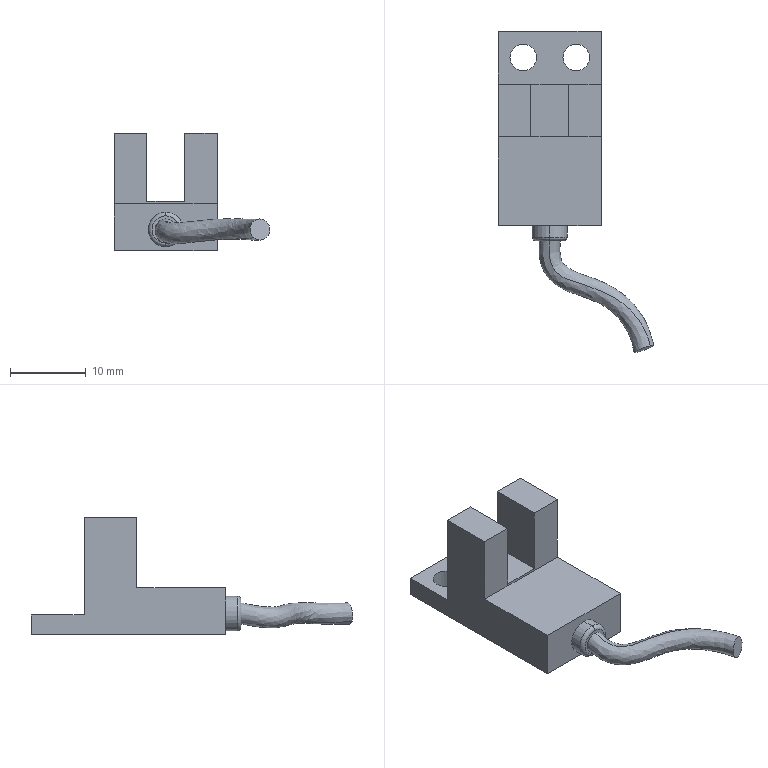Part | SolidWorks | features ICE 5, 3DProfileFeature 2, Extrusion 1, Fillet 1, Sweep 1 | 1 solid | 26 faces | box 20.544 x 42.48 x 15.5 mm | volume 2497 mm3 | plane 16 | cylinder 6 | torus 2 | spline 2 | commonest cylinder face diameters 3.5 x4 4.6 x2
STEP:
#1=CARTESIAN_POINT('',(1.75,9.375,0.));
#2=VERTEX_POINT('',#1);
#3=CARTESIAN_POINT('',(5.25,9.375,0.));
#4=VERTEX_POINT('',#3);
#5=CARTESIAN_POINT('',(3.5,9.375,0.));
#6=DIRECTION('',(0.,0.,1.));
#7=DIRECTION('',(1.,0.,0.));
#8=AXIS2_PLACEMENT_3D('',#5,#6,#7);
#9=CIRCLE('',#8,1.75);
#10=EDGE_CURVE('',#2,#4,#9,.T.);
#11=ORIENTED_EDGE('',*,*,#10,.F.);
#12=CARTESIAN_POINT('',(1.75,9.375,2.6));
#13=VERTEX_POINT('',#12);
#14=CARTESIAN_POINT('',(1.75,9.375,-7.4));
#15=DIRECTION('',(0.,0.,1.));
#16=VECTOR('',#15,1000.);
#17=LINE('',#14,#16);
#18=EDGE_CURVE('',#2,#13,#17,.T.);
#19=ORIENTED_EDGE('',*,*,#18,.T.);
#20=CARTESIAN_POINT('',(5.25,9.375,2.6));
#21=VERTEX_POINT('',#20);
#22=CARTESIAN_POINT('',(3.5,9.375,2.6));
#23=DIRECTION('',(0.,0.,1.));
#24=DIRECTION('',(-1.,0.,0.));
#25=AXIS2_PLACEMENT_3D('',#22,#23,#24);
#26=CIRCLE('',#25,1.75);
#27=EDGE_CURVE('',#13,#21,#26,.T.);
#28=ORIENTED_EDGE('',*,*,#27,.T.);
#29=CARTESIAN_POINT('',(5.25,9.375,-7.4));
#30=DIRECTION('',(0.,0.,1.));
#31=VECTOR('',#30,1000.);
#32=LINE('',#29,#31);
#33=EDGE_CURVE('',#4,#21,#32,.T.);
#34=ORIENTED_EDGE('',*,*,#33,.F.);
#35=EDGE_LOOP('',(#11,#19,#28,#34));
#36=FACE_OUTER_BOUND('',#35,.T.);
#37=CARTESIAN_POINT('',(3.5,9.375,-7.4));
#38=DIRECTION('',(0.,0.,1.));
#39=DIRECTION('',(1.,0.,0.));
#40=AXIS2_PLACEMENT_3D('',#37,#38,#39);
#41=CYLINDRICAL_SURFACE('',#40,1.75);
#42=ADVANCED_FACE('',(#36),#41,.F.);
#43=CARTESIAN_POINT('',(-5.25,9.375,0.));
#44=VERTEX_POINT('',#43);
#45=CARTESIAN_POINT('',(-1.75,9.375,0.));
#46=VERTEX_POINT('',#45);
#47=CARTESIAN_POINT('',(-3.5,9.375,0.));
#48=DIRECTION('',(0.,0.,1.));
#49=DIRECTION('',(1.,0.,0.));
#50=AXIS2_PLACEMENT_3D('',#47,#48,#49);
#51=CIRCLE('',#50,1.75);
#52=EDGE_CURVE('',#44,#46,#51,.T.);
#53=ORIENTED_EDGE('',*,*,#52,.F.);
#54=CARTESIAN_POINT('',(-5.25,9.375,2.6));
#55=VERTEX_POINT('',#54);
#56=CARTESIAN_POINT('',(-5.25,9.375,-7.4));
#57=DIRECTION('',(0.,0.,1.));
#58=VECTOR('',#57,1000.);
#59=LINE('',#56,#58);
#60=EDGE_CURVE('',#44,#55,#59,.T.);
#61=ORIENTED_EDGE('',*,*,#60,.T.);
#62=CARTESIAN_POINT('',(-1.75,9.375,2.6));
#63=VERTEX_POINT('',#62);
#64=CARTESIAN_POINT('',(-3.5,9.375,2.6));
#65=DIRECTION('',(0.,0.,1.));
#66=DIRECTION('',(1.,0.,0.));
#67=AXIS2_PLACEMENT_3D('',#64,#65,#66);
#68=CIRCLE('',#67,1.75);
#69=EDGE_CURVE('',#55,#63,#68,.T.);
#70=ORIENTED_EDGE('',*,*,#69,.T.);
#71=CARTESIAN_POINT('',(-1.75,9.375,-7.4));
#72=DIRECTION('',(0.,0.,1.));
#73=VECTOR('',#72,1000.);
#74=LINE('',#71,#73);
#75=EDGE_CURVE('',#46,#63,#74,.T.);
#76=ORIENTED_EDGE('',*,*,#75,.F.);
#77=EDGE_LOOP('',(#53,#61,#70,#76));
#78=FACE_OUTER_BOUND('',#77,.T.);
#79=CARTESIAN_POINT('',(-3.5,9.375,-7.4));
#80=DIRECTION('',(0.,0.,1.));
#81=DIRECTION('',(1.,0.,0.));
#82=AXIS2_PLACEMENT_3D('',#79,#80,#81);
#83=CYLINDRICAL_SURFACE('',#82,1.75);
#84=ADVANCED_FACE('',(#78),#83,.F.);
#85=CARTESIAN_POINT('',(0.,-14.35,5.1));
#86=VERTEX_POINT('',#85);
#87=CARTESIAN_POINT('',(0.,-14.35,0.5));
#88=VERTEX_POINT('',#87);
#89=CARTESIAN_POINT('',(0.,-14.35,2.8));
#90=DIRECTION('',(0.,1.,0.));
#91=DIRECTION('',(0.,0.,-1.));
#92=AXIS2_PLACEMENT_3D('',#89,#90,#91);
#93=CIRCLE('',#92,2.3);
#94=EDGE_CURVE('',#86,#88,#93,.T.);
#95=ORIENTED_EDGE('',*,*,#94,.F.);
#96=CARTESIAN_POINT('',(0.,-14.85,4.6));
#97=VERTEX_POINT('',#96);
#98=CARTESIAN_POINT('',(0.,-14.35,4.6));
#99=DIRECTION('',(1.,0.,0.));
#100=DIRECTION('',(0.,0.,-1.));
#101=AXIS2_PLACEMENT_3D('',#98,#99,#100);
#102=CIRCLE('',#101,0.5);
#103=EDGE_CURVE('',#86,#97,#102,.T.);
#104=ORIENTED_EDGE('',*,*,#103,.T.);
#105=CARTESIAN_POINT('',(0.,-14.85,1.));
#106=VERTEX_POINT('',#105);
#107=CARTESIAN_POINT('',(0.,-14.85,2.8));
#108=DIRECTION('',(0.,-1.,0.));
#109=DIRECTION('',(0.,0.,-1.));
#110=AXIS2_PLACEMENT_3D('',#107,#108,#109);
#111=CIRCLE('',#110,1.8);
#112=EDGE_CURVE('',#106,#97,#111,.T.);
#113=ORIENTED_EDGE('',*,*,#112,.F.);
#114=CARTESIAN_POINT('',(0.,-14.35,1.));
#115=DIRECTION('',(-1.,0.,0.));
#116=DIRECTION('',(0.,0.,1.));
#117=AXIS2_PLACEMENT_3D('',#114,#115,#116);
#118=CIRCLE('',#117,0.5);
#119=EDGE_CURVE('',#88,#106,#118,.T.);
#120=ORIENTED_EDGE('',*,*,#119,.F.);
#121=EDGE_LOOP('',(#95,#104,#113,#120));
#122=FACE_OUTER_BOUND('',#121,.T.);
#123=CARTESIAN_POINT('',(0.,-14.35,2.8));
#124=DIRECTION('',(0.,-1.,0.));
#125=DIRECTION('',(0.,0.,-1.));
#126=AXIS2_PLACEMENT_3D('',#123,#124,#125);
#127=TOROIDAL_SURFACE('',#126,1.8,0.5);
#128=ADVANCED_FACE('',(#122),#127,.T.);
#129=CARTESIAN_POINT('',(0.,-14.85,1.4));
#130=VERTEX_POINT('',#129);
#131=CARTESIAN_POINT('',(0.,-14.85,4.2));
#132=VERTEX_POINT('',#131);
#133=CARTESIAN_POINT('',(0.,-14.85,2.8));
#134=DIRECTION('',(0.,-1.,0.));
#135=DIRECTION('',(0.,0.,-1.));
#136=AXIS2_PLACEMENT_3D('',#133,#134,#135);
#137=CIRCLE('',#136,1.4);
#138=EDGE_CURVE('',#130,#132,#137,.T.);
#139=ORIENTED_EDGE('',*,*,#138,.T.);
#140=CARTESIAN_POINT('',(13.28,-28.663,3.825));
#141=VERTEX_POINT('',#140);
#142=CARTESIAN_POINT('',(0.,-14.85,4.2));
#143=CARTESIAN_POINT('',(-0.04607,-15.161,4.137));
#144=CARTESIAN_POINT('',(-0.1037,-15.745,4.024));
#145=CARTESIAN_POINT('',(-0.1038,-16.511,3.891));
#146=CARTESIAN_POINT('',(-0.02416,-17.179,3.791));
#147=CARTESIAN_POINT('',(0.1446,-17.827,3.71));
#148=CARTESIAN_POINT('',(0.4276,-18.437,3.658));
#149=CARTESIAN_POINT('',(0.8571,-18.995,3.641));
#150=CARTESIAN_POINT('',(1.754,-19.797,3.673));
#151=CARTESIAN_POINT('',(3.569,-20.261,3.835));
#152=CARTESIAN_POINT('',(5.395,-20.954,4.061));
#153=CARTESIAN_POINT('',(7.095,-21.606,4.181));
#154=CARTESIAN_POINT('',(8.774,-22.353,4.215));
#155=CARTESIAN_POINT('',(10.528,-23.728,4.109));
#156=CARTESIAN_POINT('',(11.876,-25.332,3.968));
#157=CARTESIAN_POINT('',(12.763,-26.903,3.859));
#158=CARTESIAN_POINT('',(13.142,-28.066,3.827));
#159=CARTESIAN_POINT('',(13.28,-28.663,3.825));
#160=B_SPLINE_CURVE_WITH_KNOTS('',3,(#142,#143,#144,#145,#146,#147,#148,#149,#150,#151,#152,#153,#154,#155,#156,#157,#158,#159),.UNSPECIFIED.,.F.,.F.,(4,1,1,1,1,1,1,1,1,1,1,1,1,1,1,4),(0.,0.03125,0.0625,0.09375,0.125,0.1667,0.2083,0.25,0.375,0.5,0.526,0.625,0.75,0.8333,0.9167,1.),.UNSPECIFIED.);
#161=EDGE_CURVE('',#132,#141,#160,.T.);
#162=ORIENTED_EDGE('',*,*,#161,.T.);
#163=CARTESIAN_POINT('',(11.593,-29.552,1.775));
#164=VERTEX_POINT('',#163);
#165=CARTESIAN_POINT('',(12.436,-29.108,2.8));
#166=DIRECTION('',(-0.3574,0.9277,-0.1081));
#167=DIRECTION('',(-0.9331,-0.3595,0.));
#168=AXIS2_PLACEMENT_3D('',#165,#166,#167);
#169=CIRCLE('',#168,1.4);
#170=EDGE_CURVE('',#141,#164,#169,.T.);
#171=ORIENTED_EDGE('',*,*,#170,.T.);
#172=CARTESIAN_POINT('',(0.,-14.85,1.4));
#173=CARTESIAN_POINT('',(-0.03267,-15.178,1.337));
#174=CARTESIAN_POINT('',(-0.06346,-15.795,1.225));
#175=CARTESIAN_POINT('',(-0.003443,-16.618,1.095));
#176=CARTESIAN_POINT('',(0.1547,-17.343,1.));
#177=CARTESIAN_POINT('',(0.4312,-18.046,0.9328));
#178=CARTESIAN_POINT('',(0.8497,-18.694,0.9009));
#179=CARTESIAN_POINT('',(1.414,-19.268,0.9099));
#180=CARTESIAN_POINT('',(2.497,-20.019,0.9772));
#181=CARTESIAN_POINT('',(4.195,-20.999,1.198));
#182=CARTESIAN_POINT('',(6.054,-21.475,1.381));
#183=CARTESIAN_POINT('',(7.509,-22.236,1.489));
#184=CARTESIAN_POINT('',(8.768,-23.273,1.538));
#185=CARTESIAN_POINT('',(10.032,-24.8,1.553));
#186=CARTESIAN_POINT('',(10.895,-26.453,1.583));
#187=CARTESIAN_POINT('',(11.394,-27.965,1.645));
#188=CARTESIAN_POINT('',(11.562,-29.013,1.721));
#189=CARTESIAN_POINT('',(11.593,-29.552,1.775));
#190=B_SPLINE_CURVE_WITH_KNOTS('',3,(#172,#173,#174,#175,#176,#177,#178,#179,#180,#181,#182,#183,#184,#185,#186,#187,#188,#189),.UNSPECIFIED.,.F.,.F.,(4,1,1,1,1,1,1,1,1,1,1,1,1,1,1,4),(0.,0.03125,0.0625,0.09375,0.125,0.1667,0.2083,0.25,0.375,0.5,0.526,0.625,0.75,0.8333,0.9167,1.),.UNSPECIFIED.);
#191=EDGE_CURVE('',#130,#164,#190,.T.);
#192=ORIENTED_EDGE('',*,*,#191,.F.);
#193=EDGE_LOOP('',(#139,#162,#171,#192));
#194=FACE_OUTER_BOUND('',#193,.T.);
#195=CARTESIAN_POINT('',(0.,-14.85,1.4));
#196=CARTESIAN_POINT('',(-0.03267,-15.178,1.337));
#197=CARTESIAN_POINT('',(-0.06346,-15.795,1.225));
#198=CARTESIAN_POINT('',(-0.003443,-16.618,1.095));
#199=CARTESIAN_POINT('',(0.1547,-17.343,1.));
#200=CARTESIAN_POINT('',(0.4312,-18.046,0.9328));
#201=CARTESIAN_POINT('',(0.8497,-18.694,0.9009));
#202=CARTESIAN_POINT('',(1.414,-19.268,0.9099));
#203=CARTESIAN_POINT('',(2.497,-20.019,0.9772));
#204=CARTESIAN_POINT('',(4.195,-20.999,1.198));
#205=CARTESIAN_POINT('',(6.054,-21.475,1.381));
#206=CARTESIAN_POINT('',(7.509,-22.236,1.489));
#207=CARTESIAN_POINT('',(8.768,-23.273,1.538));
#208=CARTESIAN_POINT('',(10.032,-24.8,1.553));
#209=CARTESIAN_POINT('',(10.895,-26.453,1.583));
#210=CARTESIAN_POINT('',(11.394,-27.965,1.645));
#211=CARTESIAN_POINT('',(11.562,-29.013,1.721));
#212=CARTESIAN_POINT('',(11.593,-29.552,1.775));
#213=CARTESIAN_POINT('',(2.8,-14.85,1.4));
#214=CARTESIAN_POINT('',(2.765,-15.09,1.35));
#215=CARTESIAN_POINT('',(2.73,-15.532,1.262));
#216=CARTESIAN_POINT('',(2.739,-16.023,1.173));
#217=CARTESIAN_POINT('',(2.789,-16.372,1.116));
#218=CARTESIAN_POINT('',(2.861,-16.627,1.078));
#219=CARTESIAN_POINT('',(2.942,-16.806,1.055));
#220=CARTESIAN_POINT('',(3.072,-16.994,1.027));
#221=CARTESIAN_POINT('',(3.48,-17.345,1.045));
#222=CARTESIAN_POINT('',(4.731,-18.314,0.5625));
#223=CARTESIAN_POINT('',(6.714,-18.764,1.027));
#224=CARTESIAN_POINT('',(8.493,-19.658,1.037));
#225=CARTESIAN_POINT('',(10.188,-20.94,0.7597));
#226=CARTESIAN_POINT('',(11.739,-22.857,0.4239));
#227=CARTESIAN_POINT('',(12.79,-24.973,0.1199));
#228=CARTESIAN_POINT('',(13.383,-26.926,-0.06282));
#229=CARTESIAN_POINT('',(13.557,-28.3,-0.1027));
#230=CARTESIAN_POINT('',(13.591,-29.001,-0.1076));
#231=CARTESIAN_POINT('',(2.8,-14.85,4.2));
#232=CARTESIAN_POINT('',(2.752,-15.073,4.15));
#233=CARTESIAN_POINT('',(2.69,-15.482,4.062));
#234=CARTESIAN_POINT('',(2.639,-15.916,3.97));
#235=CARTESIAN_POINT('',(2.611,-16.208,3.907));
#236=CARTESIAN_POINT('',(2.574,-16.408,3.856));
#237=CARTESIAN_POINT('',(2.52,-16.549,3.812));
#238=CARTESIAN_POINT('',(2.515,-16.72,3.758));
#239=CARTESIAN_POINT('',(2.737,-17.123,3.74));
#240=CARTESIAN_POINT('',(4.105,-17.576,3.2));
#241=CARTESIAN_POINT('',(6.056,-18.243,3.707));
#242=CARTESIAN_POINT('',(8.078,-19.028,3.729));
#243=CARTESIAN_POINT('',(10.195,-20.02,3.437));
#244=CARTESIAN_POINT('',(12.235,-21.786,2.98));
#245=CARTESIAN_POINT('',(13.772,-23.852,2.504));
#246=CARTESIAN_POINT('',(14.752,-25.864,2.152));
#247=CARTESIAN_POINT('',(15.138,-27.353,2.003));
#248=CARTESIAN_POINT('',(15.278,-28.113,1.943));
#249=CARTESIAN_POINT('',(0.,-14.85,4.2));
#250=CARTESIAN_POINT('',(-0.04607,-15.161,4.137));
#251=CARTESIAN_POINT('',(-0.1037,-15.745,4.024));
#252=CARTESIAN_POINT('',(-0.1038,-16.511,3.891));
#253=CARTESIAN_POINT('',(-0.02416,-17.179,3.791));
#254=CARTESIAN_POINT('',(0.1446,-17.827,3.71));
#255=CARTESIAN_POINT('',(0.4276,-18.437,3.658));
#256=CARTESIAN_POINT('',(0.8571,-18.995,3.641));
#257=CARTESIAN_POINT('',(1.754,-19.797,3.673));
#258=CARTESIAN_POINT('',(3.569,-20.261,3.835));
#259=CARTESIAN_POINT('',(5.395,-20.954,4.061));
#260=CARTESIAN_POINT('',(7.095,-21.606,4.181));
#261=CARTESIAN_POINT('',(8.774,-22.353,4.215));
#262=CARTESIAN_POINT('',(10.528,-23.728,4.109));
#263=CARTESIAN_POINT('',(11.876,-25.332,3.968));
#264=CARTESIAN_POINT('',(12.763,-26.903,3.859));
#265=CARTESIAN_POINT('',(13.142,-28.066,3.827));
#266=CARTESIAN_POINT('',(13.28,-28.663,3.825));
#267=CARTESIAN_POINT('',(-2.8,-14.85,4.2));
#268=CARTESIAN_POINT('',(-2.844,-15.249,4.124));
#269=CARTESIAN_POINT('',(-2.897,-16.008,3.986));
#270=CARTESIAN_POINT('',(-2.847,-17.106,3.813));
#271=CARTESIAN_POINT('',(-2.659,-18.151,3.675));
#272=CARTESIAN_POINT('',(-2.285,-19.246,3.565));
#273=CARTESIAN_POINT('',(-1.665,-20.326,3.505));
#274=CARTESIAN_POINT('',(-0.8004,-21.269,3.524));
#275=CARTESIAN_POINT('',(0.7714,-22.471,3.605));
#276=CARTESIAN_POINT('',(3.034,-22.946,4.471));
#277=CARTESIAN_POINT('',(4.735,-23.666,4.415));
#278=CARTESIAN_POINT('',(6.111,-24.184,4.633));
#279=CARTESIAN_POINT('',(7.354,-24.686,4.993));
#280=CARTESIAN_POINT('',(8.822,-25.67,5.238));
#281=CARTESIAN_POINT('',(9.981,-26.813,5.431));
#282=CARTESIAN_POINT('',(10.774,-27.942,5.566));
#283=CARTESIAN_POINT('',(11.147,-28.78,5.651));
#284=CARTESIAN_POINT('',(11.281,-29.214,5.708));
#285=CARTESIAN_POINT('',(-2.8,-14.85,1.4));
#286=CARTESIAN_POINT('',(-2.831,-15.266,1.324));
#287=CARTESIAN_POINT('',(-2.857,-16.059,1.187));
#288=CARTESIAN_POINT('',(-2.746,-17.213,1.016));
#289=CARTESIAN_POINT('',(-2.48,-18.314,0.8846));
#290=CARTESIAN_POINT('',(-1.998,-19.465,0.7875));
#291=CARTESIAN_POINT('',(-1.243,-20.582,0.7474));
#292=CARTESIAN_POINT('',(-0.2434,-21.542,0.7931));
#293=CARTESIAN_POINT('',(1.514,-22.693,0.9098));
#294=CARTESIAN_POINT('',(3.66,-23.684,1.834));
#295=CARTESIAN_POINT('',(5.393,-24.187,1.735));
#296=CARTESIAN_POINT('',(6.526,-24.814,1.941));
#297=CARTESIAN_POINT('',(7.348,-25.606,2.316));
#298=CARTESIAN_POINT('',(8.325,-26.742,2.682));
#299=CARTESIAN_POINT('',(8.999,-27.933,3.047));
#300=CARTESIAN_POINT('',(9.405,-29.004,3.352));
#301=CARTESIAN_POINT('',(9.566,-29.727,3.545));
#302=CARTESIAN_POINT('',(9.595,-30.103,3.657));
#303=CARTESIAN_POINT('',(0.,-14.85,1.4));
#304=CARTESIAN_POINT('',(-0.03267,-15.178,1.337));
#305=CARTESIAN_POINT('',(-0.06346,-15.795,1.225));
#306=CARTESIAN_POINT('',(-0.003443,-16.618,1.095));
#307=CARTESIAN_POINT('',(0.1547,-17.343,1.));
#308=CARTESIAN_POINT('',(0.4312,-18.046,0.9328));
#309=CARTESIAN_POINT('',(0.8497,-18.694,0.9009));
#310=CARTESIAN_POINT('',(1.414,-19.268,0.9099));
#311=CARTESIAN_POINT('',(2.497,-20.019,0.9772));
#312=CARTESIAN_POINT('',(4.195,-20.999,1.198));
#313=CARTESIAN_POINT('',(6.054,-21.475,1.381));
#314=CARTESIAN_POINT('',(7.509,-22.236,1.489));
#315=CARTESIAN_POINT('',(8.768,-23.273,1.538));
#316=CARTESIAN_POINT('',(10.032,-24.8,1.553));
#317=CARTESIAN_POINT('',(10.895,-26.453,1.583));
#318=CARTESIAN_POINT('',(11.394,-27.965,1.645));
#319=CARTESIAN_POINT('',(11.562,-29.013,1.721));
#320=CARTESIAN_POINT('',(11.593,-29.552,1.775));
#321=(BOUNDED_SURFACE()B_SPLINE_SURFACE(3,3,((#195,#196,#197,#198,#199,#200,#201,#202,#203,#204,#205,#206,#207,#208,#209,#210,#211,#212),(#213,#214,#215,#216,#217,#218,#219,#220,#221,#222,#223,#224,#225,#226,#227,#228,#229,#230),(#231,#232,#233,#234,#235,#236,#237,#238,#239,#240,#241,#242,#243,#244,#245,#246,#247,#248),(#249,#250,#251,#252,#253,#254,#255,#256,#257,#258,#259,#260,#261,#262,#263,#264,#265,#266),(#267,#268,#269,#270,#271,#272,#273,#274,#275,#276,#277,#278,#279,#280,#281,#282,#283,#284),(#285,#286,#287,#288,#289,#290,#291,#292,#293,#294,#295,#296,#297,#298,#299,#300,#301,#302),(#303,#304,#305,#306,#307,#308,#309,#310,#311,#312,#313,#314,#315,#316,#317,#318,#319,#320)),.UNSPECIFIED.,.T.,.F.,.T.)B_SPLINE_SURFACE_WITH_KNOTS((4,3,4),(4,1,1,1,1,1,1,1,1,1,1,1,1,1,1,4),(0.,0.5,1.),(0.,0.03125,0.0625,0.09375,0.125,0.1667,0.2083,0.25,0.375,0.5,0.526,0.625,0.75,0.8333,0.9167,1.),.UNSPECIFIED.)GEOMETRIC_REPRESENTATION_ITEM()RATIONAL_B_SPLINE_SURFACE(((1.,1.,1.,1.,1.,1.,1.,1.,1.,1.,1.,1.,1.,1.,1.,1.,1.,1.),(0.3333,0.3333,0.3333,0.3333,0.3333,0.3333,0.3333,0.3333,0.3333,0.3333,0.3333,0.3333,0.3333,0.3333,0.3333,0.3333,0.3333,0.3333),(0.3333,0.3333,0.3333,0.3333,0.3333,0.3333,0.3333,0.3333,0.3333,0.3333,0.3333,0.3333,0.3333,0.3333,0.3333,0.3333,0.3333,0.3333),(1.,1.,1.,1.,1.,1.,1.,1.,1.,1.,1.,1.,1.,1.,1.,1.,1.,1.),(0.3333,0.3333,0.3333,0.3333,0.3333,0.3333,0.3333,0.3333,0.3333,0.3333,0.3333,0.3333,0.3333,0.3333,0.3333,0.3333,0.3333,0.3333),(0.3333,0.3333,0.3333,0.3333,0.3333,0.3333,0.3333,0.3333,0.3333,0.3333,0.3333,0.3333,0.3333,0.3333,0.3333,0.3333,0.3333,0.3333),(1.,1.,1.,1.,1.,1.,1.,1.,1.,1.,1.,1.,1.,1.,1.,1.,1.,1.)))REPRESENTATION_ITEM('')SURFACE());
#322=ADVANCED_FACE('',(#194),#321,.T.);
#323=ORIENTED_EDGE('',*,*,#94,.T.);
#324=CARTESIAN_POINT('',(0.,-12.85,0.5));
#325=VERTEX_POINT('',#324);
#326=CARTESIAN_POINT('',(0.,-14.85,0.5));
#327=DIRECTION('',(0.,1.,0.));
#328=VECTOR('',#327,1000.);
#329=LINE('',#326,#328);
#330=EDGE_CURVE('',#88,#325,#329,.T.);
#331=ORIENTED_EDGE('',*,*,#330,.T.);
#332=CARTESIAN_POINT('',(0.,-12.85,5.1));
#333=VERTEX_POINT('',#332);
#334=CARTESIAN_POINT('',(0.,-12.85,2.8));
#335=DIRECTION('',(0.,-1.,0.));
#336=DIRECTION('',(0.,0.,1.));
#337=AXIS2_PLACEMENT_3D('',#334,#335,#336);
#338=CIRCLE('',#337,2.3);
#339=EDGE_CURVE('',#325,#333,#338,.T.);
#340=ORIENTED_EDGE('',*,*,#339,.T.);
#341=CARTESIAN_POINT('',(0.,-14.85,5.1));
#342=DIRECTION('',(0.,1.,0.));
#343=VECTOR('',#342,1000.);
#344=LINE('',#341,#343);
#345=EDGE_CURVE('',#86,#333,#344,.T.);
#346=ORIENTED_EDGE('',*,*,#345,.F.);
#347=EDGE_LOOP('',(#323,#331,#340,#346));
#348=FACE_OUTER_BOUND('',#347,.T.);
#349=CARTESIAN_POINT('',(0.,-14.85,2.8));
#350=DIRECTION('',(0.,1.,0.));
#351=DIRECTION('',(0.,0.,1.));
#352=AXIS2_PLACEMENT_3D('',#349,#350,#351);
#353=CYLINDRICAL_SURFACE('',#352,2.3);
#354=ADVANCED_FACE('',(#348),#353,.T.);
#355=CARTESIAN_POINT('',(6.8,-12.85,6.2));
#356=VERTEX_POINT('',#355);
#357=CARTESIAN_POINT('',(6.8,-12.85,0.));
#358=VERTEX_POINT('',#357);
#359=CARTESIAN_POINT('',(6.8,-12.85,15.5));
#360=DIRECTION('',(0.,0.,-1.));
#361=VECTOR('',#360,1000.);
#362=LINE('',#359,#361);
#363=EDGE_CURVE('',#356,#358,#362,.T.);
#364=ORIENTED_EDGE('',*,*,#363,.F.);
#365=CARTESIAN_POINT('',(-6.8,-12.85,6.2));
#366=VERTEX_POINT('',#365);
#367=CARTESIAN_POINT('',(-6.8,-12.85,6.2));
#368=DIRECTION('',(1.,0.,0.));
#369=VECTOR('',#368,1000.);
#370=LINE('',#367,#369);
#371=EDGE_CURVE('',#366,#356,#370,.T.);
#372=ORIENTED_EDGE('',*,*,#371,.F.);
#373=CARTESIAN_POINT('',(-6.8,-12.85,0.));
#374=VERTEX_POINT('',#373);
#375=CARTESIAN_POINT('',(-6.8,-12.85,15.5));
#376=DIRECTION('',(0.,0.,-1.));
#377=VECTOR('',#376,1000.);
#378=LINE('',#375,#377);
#379=EDGE_CURVE('',#366,#374,#378,.T.);
#380=ORIENTED_EDGE('',*,*,#379,.T.);
#381=CARTESIAN_POINT('',(-6.8,-12.85,0.));
#382=DIRECTION('',(1.,0.,0.));
#383=VECTOR('',#382,1000.);
#384=LINE('',#381,#383);
#385=EDGE_CURVE('',#374,#358,#384,.T.);
#386=ORIENTED_EDGE('',*,*,#385,.T.);
#387=EDGE_LOOP('',(#364,#372,#380,#386));
#388=FACE_OUTER_BOUND('',#387,.T.);
#389=CARTESIAN_POINT('',(0.,-12.85,2.8));
#390=DIRECTION('',(0.,-1.,0.));
#391=DIRECTION('',(0.,0.,1.));
#392=AXIS2_PLACEMENT_3D('',#389,#390,#391);
#393=CIRCLE('',#392,2.3);
#394=EDGE_CURVE('',#333,#325,#393,.T.);
#395=ORIENTED_EDGE('',*,*,#394,.F.);
#396=ORIENTED_EDGE('',*,*,#339,.F.);
#397=EDGE_LOOP('',(#395,#396));
#398=FACE_BOUND('',#397,.T.);
#399=CARTESIAN_POINT('',(-6.8,-12.85,15.5));
#400=DIRECTION('',(0.,1.,0.));
#401=DIRECTION('',(0.,0.,1.));
#402=AXIS2_PLACEMENT_3D('',#399,#400,#401);
#403=PLANE('',#402);
#404=ADVANCED_FACE('',(#388,#398),#403,.F.);
#405=CARTESIAN_POINT('',(-2.5,5.85,15.5));
#406=VERTEX_POINT('',#405);
#407=CARTESIAN_POINT('',(-2.5,-1.1,15.5));
#408=VERTEX_POINT('',#407);
#409=CARTESIAN_POINT('',(-2.5,-1.1,15.5));
#410=DIRECTION('',(0.,-1.,0.));
#411=VECTOR('',#410,1000.);
#412=LINE('',#409,#411);
#413=EDGE_CURVE('',#406,#408,#412,.T.);
#414=ORIENTED_EDGE('',*,*,#413,.F.);
#415=CARTESIAN_POINT('',(-6.8,5.85,15.5));
#416=VERTEX_POINT('',#415);
#417=CARTESIAN_POINT('',(-6.8,5.85,15.5));
#418=DIRECTION('',(1.,0.,0.));
#419=VECTOR('',#418,1000.);
#420=LINE('',#417,#419);
#421=EDGE_CURVE('',#416,#406,#420,.T.);
#422=ORIENTED_EDGE('',*,*,#421,.F.);
#423=CARTESIAN_POINT('',(-6.8,-1.1,15.5));
#424=VERTEX_POINT('',#423);
#425=CARTESIAN_POINT('',(-6.8,12.85,15.5));
#426=DIRECTION('',(0.,-1.,0.));
#427=VECTOR('',#426,1000.);
#428=LINE('',#425,#427);
#429=EDGE_CURVE('',#416,#424,#428,.T.);
#430=ORIENTED_EDGE('',*,*,#429,.T.);
#431=CARTESIAN_POINT('',(-6.8,-1.1,15.5));
#432=DIRECTION('',(-1.,0.,0.));
#433=VECTOR('',#432,1000.);
#434=LINE('',#431,#433);
#435=EDGE_CURVE('',#408,#424,#434,.T.);
#436=ORIENTED_EDGE('',*,*,#435,.F.);
#437=EDGE_LOOP('',(#414,#422,#430,#436));
#438=FACE_OUTER_BOUND('',#437,.T.);
#439=CARTESIAN_POINT('',(6.8,-12.85,15.5));
#440=DIRECTION('',(0.,0.,1.));
#441=DIRECTION('',(1.,0.,0.));
#442=AXIS2_PLACEMENT_3D('',#439,#440,#441);
#443=PLANE('',#442);
#444=ADVANCED_FACE('',(#438),#443,.T.);
#445=CARTESIAN_POINT('',(6.8,12.85,2.6));
#446=VERTEX_POINT('',#445);
#447=CARTESIAN_POINT('',(-6.8,12.85,2.6));
#448=VERTEX_POINT('',#447);
#449=CARTESIAN_POINT('',(-6.8,12.85,2.6));
#450=DIRECTION('',(-1.,0.,0.));
#451=VECTOR('',#450,1000.);
#452=LINE('',#449,#451);
#453=EDGE_CURVE('',#446,#448,#452,.T.);
#454=ORIENTED_EDGE('',*,*,#453,.F.);
#455=CARTESIAN_POINT('',(6.8,12.85,0.));
#456=VERTEX_POINT('',#455);
#457=CARTESIAN_POINT('',(6.8,12.85,15.5));
#458=DIRECTION('',(0.,0.,-1.));
#459=VECTOR('',#458,1000.);
#460=LINE('',#457,#459);
#461=EDGE_CURVE('',#446,#456,#460,.T.);
#462=ORIENTED_EDGE('',*,*,#461,.T.);
#463=CARTESIAN_POINT('',(-6.8,12.85,0.));
#464=VERTEX_POINT('',#463);
#465=CARTESIAN_POINT('',(-6.8,12.85,0.));
#466=DIRECTION('',(-1.,0.,0.));
#467=VECTOR('',#466,1000.);
#468=LINE('',#465,#467);
#469=EDGE_CURVE('',#456,#464,#468,.T.);
#470=ORIENTED_EDGE('',*,*,#469,.T.);
#471=CARTESIAN_POINT('',(-6.8,12.85,15.5));
#472=DIRECTION('',(0.,0.,-1.));
#473=VECTOR('',#472,1000.);
#474=LINE('',#471,#473);
#475=EDGE_CURVE('',#448,#464,#474,.T.);
#476=ORIENTED_EDGE('',*,*,#475,.F.);
#477=EDGE_LOOP('',(#454,#462,#470,#476));
#478=FACE_OUTER_BOUND('',#477,.T.);
#479=CARTESIAN_POINT('',(-6.8,12.85,15.5));
#480=DIRECTION('',(0.,-1.,0.));
#481=DIRECTION('',(0.,0.,-1.));
#482=AXIS2_PLACEMENT_3D('',#479,#480,#481);
#483=PLANE('',#482);
#484=ADVANCED_FACE('',(#478),#483,.F.);
#485=CARTESIAN_POINT('',(6.8,-1.1,15.5));
#486=VERTEX_POINT('',#485);
#487=CARTESIAN_POINT('',(6.8,5.85,15.5));
#488=VERTEX_POINT('',#487);
#489=CARTESIAN_POINT('',(6.8,12.85,15.5));
#490=DIRECTION('',(0.,1.,0.));
#491=VECTOR('',#490,1000.);
#492=LINE('',#489,#491);
#493=EDGE_CURVE('',#486,#488,#492,.T.);
#494=ORIENTED_EDGE('',*,*,#493,.F.);
#495=CARTESIAN_POINT('',(6.8,-1.1,6.2));
#496=VERTEX_POINT('',#495);
#497=CARTESIAN_POINT('',(6.8,-1.1,6.2));
#498=DIRECTION('',(0.,0.,1.));
#499=VECTOR('',#498,1000.);
#500=LINE('',#497,#499);
#501=EDGE_CURVE('',#496,#486,#500,.T.);
#502=ORIENTED_EDGE('',*,*,#501,.F.);
#503=CARTESIAN_POINT('',(6.8,-12.85,6.2));
#504=DIRECTION('',(0.,1.,0.));
#505=VECTOR('',#504,1000.);
#506=LINE('',#503,#505);
#507=EDGE_CURVE('',#356,#496,#506,.T.);
#508=ORIENTED_EDGE('',*,*,#507,.F.);
#509=ORIENTED_EDGE('',*,*,#363,.T.);
#510=CARTESIAN_POINT('',(6.8,12.85,0.));
#511=DIRECTION('',(0.,1.,0.));
#512=VECTOR('',#511,1000.);
#513=LINE('',#510,#512);
#514=EDGE_CURVE('',#358,#456,#513,.T.);
#515=ORIENTED_EDGE('',*,*,#514,.T.);
#516=ORIENTED_EDGE('',*,*,#461,.F.);
#517=CARTESIAN_POINT('',(6.8,5.85,2.6));
#518=VERTEX_POINT('',#517);
#519=CARTESIAN_POINT('',(6.8,12.85,2.6));
#520=DIRECTION('',(0.,1.,0.));
#521=VECTOR('',#520,1000.);
#522=LINE('',#519,#521);
#523=EDGE_CURVE('',#518,#446,#522,.T.);
#524=ORIENTED_EDGE('',*,*,#523,.F.);
#525=CARTESIAN_POINT('',(6.8,5.85,2.6));
#526=DIRECTION('',(0.,0.,1.));
#527=VECTOR('',#526,1000.);
#528=LINE('',#525,#527);
#529=EDGE_CURVE('',#518,#488,#528,.T.);
#530=ORIENTED_EDGE('',*,*,#529,.T.);
#531=EDGE_LOOP('',(#494,#502,#508,#509,#515,#516,#524,#530));
#532=FACE_OUTER_BOUND('',#531,.T.);
#533=CARTESIAN_POINT('',(6.8,12.85,15.5));
#534=DIRECTION('',(-1.,0.,0.));
#535=DIRECTION('',(0.,-1.,0.));
#536=AXIS2_PLACEMENT_3D('',#533,#534,#535);
#537=PLANE('',#536);
#538=ADVANCED_FACE('',(#532),#537,.F.);
#539=CARTESIAN_POINT('',(-6.8,-1.1,6.2));
#540=VERTEX_POINT('',#539);
#541=CARTESIAN_POINT('',(-6.8,-12.85,6.2));
#542=DIRECTION('',(0.,-1.,0.));
#543=VECTOR('',#542,1000.);
#544=LINE('',#541,#543);
#545=EDGE_CURVE('',#540,#366,#544,.T.);
#546=ORIENTED_EDGE('',*,*,#545,.F.);
#547=CARTESIAN_POINT('',(-6.8,-1.1,6.2));
#548=DIRECTION('',(0.,0.,1.));
#549=VECTOR('',#548,1000.);
#550=LINE('',#547,#549);
#551=EDGE_CURVE('',#540,#424,#550,.T.);
#552=ORIENTED_EDGE('',*,*,#551,.T.);
#553=ORIENTED_EDGE('',*,*,#429,.F.);
#554=CARTESIAN_POINT('',(-6.8,5.85,2.6));
#555=VERTEX_POINT('',#554);
#556=CARTESIAN_POINT('',(-6.8,5.85,2.6));
#557=DIRECTION('',(0.,0.,1.));
#558=VECTOR('',#557,1000.);
#559=LINE('',#556,#558);
#560=EDGE_CURVE('',#555,#416,#559,.T.);
#561=ORIENTED_EDGE('',*,*,#560,.F.);
#562=CARTESIAN_POINT('',(-6.8,12.85,2.6));
#563=DIRECTION('',(0.,-1.,0.));
#564=VECTOR('',#563,1000.);
#565=LINE('',#562,#564);
#566=EDGE_CURVE('',#448,#555,#565,.T.);
#567=ORIENTED_EDGE('',*,*,#566,.F.);
#568=ORIENTED_EDGE('',*,*,#475,.T.);
#569=CARTESIAN_POINT('',(-6.8,12.85,0.));
#570=DIRECTION('',(0.,-1.,0.));
#571=VECTOR('',#570,1000.);
#572=LINE('',#569,#571);
#573=EDGE_CURVE('',#464,#374,#572,.T.);
#574=ORIENTED_EDGE('',*,*,#573,.T.);
#575=ORIENTED_EDGE('',*,*,#379,.F.);
#576=EDGE_LOOP('',(#546,#552,#553,#561,#567,#568,#574,#575));
#577=FACE_OUTER_BOUND('',#576,.T.);
#578=CARTESIAN_POINT('',(-6.8,12.85,15.5));
#579=DIRECTION('',(1.,0.,0.));
#580=DIRECTION('',(0.,1.,0.));
#581=AXIS2_PLACEMENT_3D('',#578,#579,#580);
#582=PLANE('',#581);
#583=ADVANCED_FACE('',(#577),#582,.F.);
#584=CARTESIAN_POINT('',(2.5,-1.1,15.5));
#585=VERTEX_POINT('',#584);
#586=CARTESIAN_POINT('',(2.5,5.85,15.5));
#587=VERTEX_POINT('',#586);
#588=CARTESIAN_POINT('',(2.5,-1.1,15.5));
#589=DIRECTION('',(0.,1.,0.));
#590=VECTOR('',#589,1000.);
#591=LINE('',#588,#590);
#592=EDGE_CURVE('',#585,#587,#591,.T.);
#593=ORIENTED_EDGE('',*,*,#592,.F.);
#594=CARTESIAN_POINT('',(-6.8,-1.1,15.5));
#595=DIRECTION('',(-1.,0.,0.));
#596=VECTOR('',#595,1000.);
#597=LINE('',#594,#596);
#598=EDGE_CURVE('',#486,#585,#597,.T.);
#599=ORIENTED_EDGE('',*,*,#598,.F.);
#600=ORIENTED_EDGE('',*,*,#493,.T.);
#601=CARTESIAN_POINT('',(-6.8,5.85,15.5));
#602=DIRECTION('',(1.,0.,0.));
#603=VECTOR('',#602,1000.);
#604=LINE('',#601,#603);
#605=EDGE_CURVE('',#587,#488,#604,.T.);
#606=ORIENTED_EDGE('',*,*,#605,.F.);
#607=EDGE_LOOP('',(#593,#599,#600,#606));
#608=FACE_OUTER_BOUND('',#607,.T.);
#609=CARTESIAN_POINT('',(6.8,-12.85,15.5));
#610=DIRECTION('',(0.,0.,1.));
#611=DIRECTION('',(1.,0.,0.));
#612=AXIS2_PLACEMENT_3D('',#609,#610,#611);
#613=PLANE('',#612);
#614=ADVANCED_FACE('',(#608),#613,.T.);
#615=CARTESIAN_POINT('',(3.5,9.375,0.));
#616=DIRECTION('',(0.,0.,1.));
#617=DIRECTION('',(1.,0.,0.));
#618=AXIS2_PLACEMENT_3D('',#615,#616,#617);
#619=CIRCLE('',#618,1.75);
#620=EDGE_CURVE('',#4,#2,#619,.T.);
#621=ORIENTED_EDGE('',*,*,#620,.T.);
#622=ORIENTED_EDGE('',*,*,#10,.T.);
#623=EDGE_LOOP('',(#621,#622));
#624=FACE_BOUND('',#623,.T.);
#625=CARTESIAN_POINT('',(-3.5,9.375,0.));
#626=DIRECTION('',(0.,0.,1.));
#627=DIRECTION('',(1.,0.,0.));
#628=AXIS2_PLACEMENT_3D('',#625,#626,#627);
#629=CIRCLE('',#628,1.75);
#630=EDGE_CURVE('',#46,#44,#629,.T.);
#631=ORIENTED_EDGE('',*,*,#630,.T.);
#632=ORIENTED_EDGE('',*,*,#52,.T.);
#633=EDGE_LOOP('',(#631,#632));
#634=FACE_BOUND('',#633,.T.);
#635=ORIENTED_EDGE('',*,*,#514,.F.);
#636=ORIENTED_EDGE('',*,*,#385,.F.);
#637=ORIENTED_EDGE('',*,*,#573,.F.);
#638=ORIENTED_EDGE('',*,*,#469,.F.);
#639=EDGE_LOOP('',(#635,#636,#637,#638));
#640=FACE_OUTER_BOUND('',#639,.T.);
#641=CARTESIAN_POINT('',(6.8,-12.85,0.));
#642=DIRECTION('',(0.,0.,1.));
#643=DIRECTION('',(1.,0.,0.));
#644=AXIS2_PLACEMENT_3D('',#641,#642,#643);
#645=PLANE('',#644);
#646=ADVANCED_FACE('',(#624,#634,#640),#645,.F.);
#647=ORIENTED_EDGE('',*,*,#421,.T.);
#648=CARTESIAN_POINT('',(-2.5,5.85,6.5));
#649=VERTEX_POINT('',#648);
#650=CARTESIAN_POINT('',(-2.5,5.85,6.5));
#651=DIRECTION('',(0.,0.,1.));
#652=VECTOR('',#651,1000.);
#653=LINE('',#650,#652);
#654=EDGE_CURVE('',#649,#406,#653,.T.);
#655=ORIENTED_EDGE('',*,*,#654,.F.);
#656=CARTESIAN_POINT('',(2.5,5.85,6.5));
#657=VERTEX_POINT('',#656);
#658=CARTESIAN_POINT('',(-2.5,5.85,6.5));
#659=DIRECTION('',(-1.,0.,0.));
#660=VECTOR('',#659,1000.);
#661=LINE('',#658,#660);
#662=EDGE_CURVE('',#657,#649,#661,.T.);
#663=ORIENTED_EDGE('',*,*,#662,.F.);
#664=CARTESIAN_POINT('',(2.5,5.85,6.5));
#665=DIRECTION('',(0.,0.,1.));
#666=VECTOR('',#665,1000.);
#667=LINE('',#664,#666);
#668=EDGE_CURVE('',#657,#587,#667,.T.);
#669=ORIENTED_EDGE('',*,*,#668,.T.);
#670=ORIENTED_EDGE('',*,*,#605,.T.);
#671=ORIENTED_EDGE('',*,*,#529,.F.);
#672=CARTESIAN_POINT('',(-6.8,5.85,2.6));
#673=DIRECTION('',(1.,0.,0.));
#674=VECTOR('',#673,1000.);
#675=LINE('',#672,#674);
#676=EDGE_CURVE('',#555,#518,#675,.T.);
#677=ORIENTED_EDGE('',*,*,#676,.F.);
#678=ORIENTED_EDGE('',*,*,#560,.T.);
#679=EDGE_LOOP('',(#647,#655,#663,#669,#670,#671,#677,#678));
#680=FACE_OUTER_BOUND('',#679,.T.);
#681=CARTESIAN_POINT('',(-6.8,5.85,2.6));
#682=DIRECTION('',(0.,-1.,0.));
#683=DIRECTION('',(0.,0.,-1.));
#684=AXIS2_PLACEMENT_3D('',#681,#682,#683);
#685=PLANE('',#684);
#686=ADVANCED_FACE('',(#680),#685,.F.);
#687=CARTESIAN_POINT('',(3.5,9.375,2.6));
#688=DIRECTION('',(0.,0.,1.));
#689=DIRECTION('',(-1.,0.,0.));
#690=AXIS2_PLACEMENT_3D('',#687,#688,#689);
#691=CIRCLE('',#690,1.75);
#692=EDGE_CURVE('',#21,#13,#691,.T.);
#693=ORIENTED_EDGE('',*,*,#692,.F.);
#694=ORIENTED_EDGE('',*,*,#27,.F.);
#695=EDGE_LOOP('',(#693,#694));
#696=FACE_BOUND('',#695,.T.);
#697=CARTESIAN_POINT('',(-3.5,9.375,2.6));
#698=DIRECTION('',(0.,0.,1.));
#699=DIRECTION('',(1.,0.,0.));
#700=AXIS2_PLACEMENT_3D('',#697,#698,#699);
#701=CIRCLE('',#700,1.75);
#702=EDGE_CURVE('',#63,#55,#701,.T.);
#703=ORIENTED_EDGE('',*,*,#702,.F.);
#704=ORIENTED_EDGE('',*,*,#69,.F.);
#705=EDGE_LOOP('',(#703,#704));
#706=FACE_BOUND('',#705,.T.);
#707=ORIENTED_EDGE('',*,*,#566,.T.);
#708=ORIENTED_EDGE('',*,*,#676,.T.);
#709=ORIENTED_EDGE('',*,*,#523,.T.);
#710=ORIENTED_EDGE('',*,*,#453,.T.);
#711=EDGE_LOOP('',(#707,#708,#709,#710));
#712=FACE_OUTER_BOUND('',#711,.T.);
#713=CARTESIAN_POINT('',(-6.8,5.85,2.6));
#714=DIRECTION('',(0.,0.,1.));
#715=DIRECTION('',(1.,0.,0.));
#716=AXIS2_PLACEMENT_3D('',#713,#714,#715);
#717=PLANE('',#716);
#718=ADVANCED_FACE('',(#696,#706,#712),#717,.T.);
#719=CARTESIAN_POINT('',(-2.5,-1.1,6.5));
#720=VERTEX_POINT('',#719);
#721=CARTESIAN_POINT('',(2.5,-1.1,6.5));
#722=VERTEX_POINT('',#721);
#723=CARTESIAN_POINT('',(-2.5,-1.1,6.5));
#724=DIRECTION('',(1.,0.,0.));
#725=VECTOR('',#724,1000.);
#726=LINE('',#723,#725);
#727=EDGE_CURVE('',#720,#722,#726,.T.);
#728=ORIENTED_EDGE('',*,*,#727,.F.);
#729=CARTESIAN_POINT('',(-2.5,-1.1,6.5));
#730=DIRECTION('',(0.,0.,1.));
#731=VECTOR('',#730,1000.);
#732=LINE('',#729,#731);
#733=EDGE_CURVE('',#720,#408,#732,.T.);
#734=ORIENTED_EDGE('',*,*,#733,.T.);
#735=ORIENTED_EDGE('',*,*,#435,.T.);
#736=ORIENTED_EDGE('',*,*,#551,.F.);
#737=CARTESIAN_POINT('',(-6.8,-1.1,6.2));
#738=DIRECTION('',(-1.,0.,0.));
#739=VECTOR('',#738,1000.);
#740=LINE('',#737,#739);
#741=EDGE_CURVE('',#496,#540,#740,.T.);
#742=ORIENTED_EDGE('',*,*,#741,.F.);
#743=ORIENTED_EDGE('',*,*,#501,.T.);
#744=ORIENTED_EDGE('',*,*,#598,.T.);
#745=CARTESIAN_POINT('',(2.5,-1.1,6.5));
#746=DIRECTION('',(0.,0.,1.));
#747=VECTOR('',#746,1000.);
#748=LINE('',#745,#747);
#749=EDGE_CURVE('',#722,#585,#748,.T.);
#750=ORIENTED_EDGE('',*,*,#749,.F.);
#751=EDGE_LOOP('',(#728,#734,#735,#736,#742,#743,#744,#750));
#752=FACE_OUTER_BOUND('',#751,.T.);
#753=CARTESIAN_POINT('',(-6.8,-1.1,6.2));
#754=DIRECTION('',(0.,1.,0.));
#755=DIRECTION('',(0.,0.,1.));
#756=AXIS2_PLACEMENT_3D('',#753,#754,#755);
#757=PLANE('',#756);
#758=ADVANCED_FACE('',(#752),#757,.F.);
#759=ORIENTED_EDGE('',*,*,#545,.T.);
#760=ORIENTED_EDGE('',*,*,#371,.T.);
#761=ORIENTED_EDGE('',*,*,#507,.T.);
#762=ORIENTED_EDGE('',*,*,#741,.T.);
#763=EDGE_LOOP('',(#759,#760,#761,#762));
#764=FACE_OUTER_BOUND('',#763,.T.);
#765=CARTESIAN_POINT('',(-6.8,-1.1,6.2));
#766=DIRECTION('',(0.,0.,-1.));
#767=DIRECTION('',(-1.,0.,0.));
#768=AXIS2_PLACEMENT_3D('',#765,#766,#767);
#769=PLANE('',#768);
#770=ADVANCED_FACE('',(#764),#769,.F.);
#771=ORIENTED_EDGE('',*,*,#413,.T.);
#772=ORIENTED_EDGE('',*,*,#733,.F.);
#773=CARTESIAN_POINT('',(-2.5,-1.1,6.5));
#774=DIRECTION('',(0.,-1.,0.));
#775=VECTOR('',#774,1000.);
#776=LINE('',#773,#775);
#777=EDGE_CURVE('',#649,#720,#776,.T.);
#778=ORIENTED_EDGE('',*,*,#777,.F.);
#779=ORIENTED_EDGE('',*,*,#654,.T.);
#780=EDGE_LOOP('',(#771,#772,#778,#779));
#781=FACE_OUTER_BOUND('',#780,.T.);
#782=CARTESIAN_POINT('',(-2.5,-1.1,6.5));
#783=DIRECTION('',(-1.,0.,0.));
#784=DIRECTION('',(0.,-1.,0.));
#785=AXIS2_PLACEMENT_3D('',#782,#783,#784);
#786=PLANE('',#785);
#787=ADVANCED_FACE('',(#781),#786,.F.);
#788=ORIENTED_EDGE('',*,*,#592,.T.);
#789=ORIENTED_EDGE('',*,*,#668,.F.);
#790=CARTESIAN_POINT('',(2.5,-1.1,6.5));
#791=DIRECTION('',(0.,1.,0.));
#792=VECTOR('',#791,1000.);
#793=LINE('',#790,#792);
#794=EDGE_CURVE('',#722,#657,#793,.T.);
#795=ORIENTED_EDGE('',*,*,#794,.F.);
#796=ORIENTED_EDGE('',*,*,#749,.T.);
#797=EDGE_LOOP('',(#788,#789,#795,#796));
#798=FACE_OUTER_BOUND('',#797,.T.);
#799=CARTESIAN_POINT('',(2.5,-1.1,6.5));
#800=DIRECTION('',(1.,0.,0.));
#801=DIRECTION('',(0.,1.,0.));
#802=AXIS2_PLACEMENT_3D('',#799,#800,#801);
#803=PLANE('',#802);
#804=ADVANCED_FACE('',(#798),#803,.F.);
#805=ORIENTED_EDGE('',*,*,#777,.T.);
#806=ORIENTED_EDGE('',*,*,#727,.T.);
#807=ORIENTED_EDGE('',*,*,#794,.T.);
#808=ORIENTED_EDGE('',*,*,#662,.T.);
#809=EDGE_LOOP('',(#805,#806,#807,#808));
#810=FACE_OUTER_BOUND('',#809,.T.);
#811=CARTESIAN_POINT('',(-2.5,5.85,6.5));
#812=DIRECTION('',(0.,0.,-1.));
#813=DIRECTION('',(-1.,0.,0.));
#814=AXIS2_PLACEMENT_3D('',#811,#812,#813);
#815=PLANE('',#814);
#816=ADVANCED_FACE('',(#810),#815,.F.);
#817=ORIENTED_EDGE('',*,*,#330,.F.);
#818=CARTESIAN_POINT('',(0.,-14.35,2.8));
#819=DIRECTION('',(0.,1.,0.));
#820=DIRECTION('',(0.,0.,-1.));
#821=AXIS2_PLACEMENT_3D('',#818,#819,#820);
#822=CIRCLE('',#821,2.3);
#823=EDGE_CURVE('',#88,#86,#822,.T.);
#824=ORIENTED_EDGE('',*,*,#823,.T.);
#825=ORIENTED_EDGE('',*,*,#345,.T.);
#826=ORIENTED_EDGE('',*,*,#394,.T.);
#827=EDGE_LOOP('',(#817,#824,#825,#826));
#828=FACE_OUTER_BOUND('',#827,.T.);
#829=CARTESIAN_POINT('',(0.,-14.85,2.8));
#830=DIRECTION('',(0.,1.,0.));
#831=DIRECTION('',(0.,0.,1.));
#832=AXIS2_PLACEMENT_3D('',#829,#830,#831);
#833=CYLINDRICAL_SURFACE('',#832,2.3);
#834=ADVANCED_FACE('',(#828),#833,.T.);
#835=ORIENTED_EDGE('',*,*,#112,.T.);
#836=CARTESIAN_POINT('',(0.,-14.85,2.8));
#837=DIRECTION('',(0.,-1.,0.));
#838=DIRECTION('',(0.,0.,-1.));
#839=AXIS2_PLACEMENT_3D('',#836,#837,#838);
#840=CIRCLE('',#839,1.8);
#841=EDGE_CURVE('',#97,#106,#840,.T.);
#842=ORIENTED_EDGE('',*,*,#841,.T.);
#843=EDGE_LOOP('',(#835,#842));
#844=FACE_OUTER_BOUND('',#843,.T.);
#845=ORIENTED_EDGE('',*,*,#138,.F.);
#846=CARTESIAN_POINT('',(0.,-14.85,2.8));
#847=DIRECTION('',(0.,-1.,0.));
#848=DIRECTION('',(0.,0.,-1.));
#849=AXIS2_PLACEMENT_3D('',#846,#847,#848);
#850=CIRCLE('',#849,1.4);
#851=EDGE_CURVE('',#132,#130,#850,.T.);
#852=ORIENTED_EDGE('',*,*,#851,.F.);
#853=EDGE_LOOP('',(#845,#852));
#854=FACE_BOUND('',#853,.T.);
#855=CARTESIAN_POINT('',(0.,-14.85,2.8));
#856=DIRECTION('',(0.,-1.,0.));
#857=DIRECTION('',(0.,0.,-1.));
#858=AXIS2_PLACEMENT_3D('',#855,#856,#857);
#859=PLANE('',#858);
#860=ADVANCED_FACE('',(#844,#854),#859,.T.);
#861=ORIENTED_EDGE('',*,*,#161,.F.);
#862=ORIENTED_EDGE('',*,*,#851,.T.);
#863=ORIENTED_EDGE('',*,*,#191,.T.);
#864=CARTESIAN_POINT('',(12.436,-29.108,2.8));
#865=DIRECTION('',(-0.3574,0.9277,-0.1081));
#866=DIRECTION('',(-0.9331,-0.3595,0.));
#867=AXIS2_PLACEMENT_3D('',#864,#865,#866);
#868=CIRCLE('',#867,1.4);
#869=EDGE_CURVE('',#164,#141,#868,.T.);
#870=ORIENTED_EDGE('',*,*,#869,.T.);
#871=EDGE_LOOP('',(#861,#862,#863,#870));
#872=FACE_OUTER_BOUND('',#871,.T.);
#873=CARTESIAN_POINT('',(0.,-14.85,1.4));
#874=CARTESIAN_POINT('',(-0.03267,-15.178,1.337));
#875=CARTESIAN_POINT('',(-0.06346,-15.795,1.225));
#876=CARTESIAN_POINT('',(-0.003443,-16.618,1.095));
#877=CARTESIAN_POINT('',(0.1547,-17.343,1.));
#878=CARTESIAN_POINT('',(0.4312,-18.046,0.9328));
#879=CARTESIAN_POINT('',(0.8497,-18.694,0.9009));
#880=CARTESIAN_POINT('',(1.414,-19.268,0.9099));
#881=CARTESIAN_POINT('',(2.497,-20.019,0.9772));
#882=CARTESIAN_POINT('',(4.195,-20.999,1.198));
#883=CARTESIAN_POINT('',(6.054,-21.475,1.381));
#884=CARTESIAN_POINT('',(7.509,-22.236,1.489));
#885=CARTESIAN_POINT('',(8.768,-23.273,1.538));
#886=CARTESIAN_POINT('',(10.032,-24.8,1.553));
#887=CARTESIAN_POINT('',(10.895,-26.453,1.583));
#888=CARTESIAN_POINT('',(11.394,-27.965,1.645));
#889=CARTESIAN_POINT('',(11.562,-29.013,1.721));
#890=CARTESIAN_POINT('',(11.593,-29.552,1.775));
#891=CARTESIAN_POINT('',(2.8,-14.85,1.4));
#892=CARTESIAN_POINT('',(2.765,-15.09,1.35));
#893=CARTESIAN_POINT('',(2.73,-15.532,1.262));
#894=CARTESIAN_POINT('',(2.739,-16.023,1.173));
#895=CARTESIAN_POINT('',(2.789,-16.372,1.116));
#896=CARTESIAN_POINT('',(2.861,-16.627,1.078));
#897=CARTESIAN_POINT('',(2.942,-16.806,1.055));
#898=CARTESIAN_POINT('',(3.072,-16.994,1.027));
#899=CARTESIAN_POINT('',(3.48,-17.345,1.045));
#900=CARTESIAN_POINT('',(4.731,-18.314,0.5625));
#901=CARTESIAN_POINT('',(6.714,-18.764,1.027));
#902=CARTESIAN_POINT('',(8.493,-19.658,1.037));
#903=CARTESIAN_POINT('',(10.188,-20.94,0.7597));
#904=CARTESIAN_POINT('',(11.739,-22.857,0.4239));
#905=CARTESIAN_POINT('',(12.79,-24.973,0.1199));
#906=CARTESIAN_POINT('',(13.383,-26.926,-0.06282));
#907=CARTESIAN_POINT('',(13.557,-28.3,-0.1027));
#908=CARTESIAN_POINT('',(13.591,-29.001,-0.1076));
#909=CARTESIAN_POINT('',(2.8,-14.85,4.2));
#910=CARTESIAN_POINT('',(2.752,-15.073,4.15));
#911=CARTESIAN_POINT('',(2.69,-15.482,4.062));
#912=CARTESIAN_POINT('',(2.639,-15.916,3.97));
#913=CARTESIAN_POINT('',(2.611,-16.208,3.907));
#914=CARTESIAN_POINT('',(2.574,-16.408,3.856));
#915=CARTESIAN_POINT('',(2.52,-16.549,3.812));
#916=CARTESIAN_POINT('',(2.515,-16.72,3.758));
#917=CARTESIAN_POINT('',(2.737,-17.123,3.74));
#918=CARTESIAN_POINT('',(4.105,-17.576,3.2));
#919=CARTESIAN_POINT('',(6.056,-18.243,3.707));
#920=CARTESIAN_POINT('',(8.078,-19.028,3.729));
#921=CARTESIAN_POINT('',(10.195,-20.02,3.437));
#922=CARTESIAN_POINT('',(12.235,-21.786,2.98));
#923=CARTESIAN_POINT('',(13.772,-23.852,2.504));
#924=CARTESIAN_POINT('',(14.752,-25.864,2.152));
#925=CARTESIAN_POINT('',(15.138,-27.353,2.003));
#926=CARTESIAN_POINT('',(15.278,-28.113,1.943));
#927=CARTESIAN_POINT('',(0.,-14.85,4.2));
#928=CARTESIAN_POINT('',(-0.04607,-15.161,4.137));
#929=CARTESIAN_POINT('',(-0.1037,-15.745,4.024));
#930=CARTESIAN_POINT('',(-0.1038,-16.511,3.891));
#931=CARTESIAN_POINT('',(-0.02416,-17.179,3.791));
#932=CARTESIAN_POINT('',(0.1446,-17.827,3.71));
#933=CARTESIAN_POINT('',(0.4276,-18.437,3.658));
#934=CARTESIAN_POINT('',(0.8571,-18.995,3.641));
#935=CARTESIAN_POINT('',(1.754,-19.797,3.673));
#936=CARTESIAN_POINT('',(3.569,-20.261,3.835));
#937=CARTESIAN_POINT('',(5.395,-20.954,4.061));
#938=CARTESIAN_POINT('',(7.095,-21.606,4.181));
#939=CARTESIAN_POINT('',(8.774,-22.353,4.215));
#940=CARTESIAN_POINT('',(10.528,-23.728,4.109));
#941=CARTESIAN_POINT('',(11.876,-25.332,3.968));
#942=CARTESIAN_POINT('',(12.763,-26.903,3.859));
#943=CARTESIAN_POINT('',(13.142,-28.066,3.827));
#944=CARTESIAN_POINT('',(13.28,-28.663,3.825));
#945=CARTESIAN_POINT('',(-2.8,-14.85,4.2));
#946=CARTESIAN_POINT('',(-2.844,-15.249,4.124));
#947=CARTESIAN_POINT('',(-2.897,-16.008,3.986));
#948=CARTESIAN_POINT('',(-2.847,-17.106,3.813));
#949=CARTESIAN_POINT('',(-2.659,-18.151,3.675));
#950=CARTESIAN_POINT('',(-2.285,-19.246,3.565));
#951=CARTESIAN_POINT('',(-1.665,-20.326,3.505));
#952=CARTESIAN_POINT('',(-0.8004,-21.269,3.524));
#953=CARTESIAN_POINT('',(0.7714,-22.471,3.605));
#954=CARTESIAN_POINT('',(3.034,-22.946,4.471));
#955=CARTESIAN_POINT('',(4.735,-23.666,4.415));
#956=CARTESIAN_POINT('',(6.111,-24.184,4.633));
#957=CARTESIAN_POINT('',(7.354,-24.686,4.993));
#958=CARTESIAN_POINT('',(8.822,-25.67,5.238));
#959=CARTESIAN_POINT('',(9.981,-26.813,5.431));
#960=CARTESIAN_POINT('',(10.774,-27.942,5.566));
#961=CARTESIAN_POINT('',(11.147,-28.78,5.651));
#962=CARTESIAN_POINT('',(11.281,-29.214,5.708));
#963=CARTESIAN_POINT('',(-2.8,-14.85,1.4));
#964=CARTESIAN_POINT('',(-2.831,-15.266,1.324));
#965=CARTESIAN_POINT('',(-2.857,-16.059,1.187));
#966=CARTESIAN_POINT('',(-2.746,-17.213,1.016));
#967=CARTESIAN_POINT('',(-2.48,-18.314,0.8846));
#968=CARTESIAN_POINT('',(-1.998,-19.465,0.7875));
#969=CARTESIAN_POINT('',(-1.243,-20.582,0.7474));
#970=CARTESIAN_POINT('',(-0.2434,-21.542,0.7931));
#971=CARTESIAN_POINT('',(1.514,-22.693,0.9098));
#972=CARTESIAN_POINT('',(3.66,-23.684,1.834));
#973=CARTESIAN_POINT('',(5.393,-24.187,1.735));
#974=CARTESIAN_POINT('',(6.526,-24.814,1.941));
#975=CARTESIAN_POINT('',(7.348,-25.606,2.316));
#976=CARTESIAN_POINT('',(8.325,-26.742,2.682));
#977=CARTESIAN_POINT('',(8.999,-27.933,3.047));
#978=CARTESIAN_POINT('',(9.405,-29.004,3.352));
#979=CARTESIAN_POINT('',(9.566,-29.727,3.545));
#980=CARTESIAN_POINT('',(9.595,-30.103,3.657));
#981=CARTESIAN_POINT('',(0.,-14.85,1.4));
#982=CARTESIAN_POINT('',(-0.03267,-15.178,1.337));
#983=CARTESIAN_POINT('',(-0.06346,-15.795,1.225));
#984=CARTESIAN_POINT('',(-0.003443,-16.618,1.095));
#985=CARTESIAN_POINT('',(0.1547,-17.343,1.));
#986=CARTESIAN_POINT('',(0.4312,-18.046,0.9328));
#987=CARTESIAN_POINT('',(0.8497,-18.694,0.9009));
#988=CARTESIAN_POINT('',(1.414,-19.268,0.9099));
#989=CARTESIAN_POINT('',(2.497,-20.019,0.9772));
#990=CARTESIAN_POINT('',(4.195,-20.999,1.198));
#991=CARTESIAN_POINT('',(6.054,-21.475,1.381));
#992=CARTESIAN_POINT('',(7.509,-22.236,1.489));
#993=CARTESIAN_POINT('',(8.768,-23.273,1.538));
#994=CARTESIAN_POINT('',(10.032,-24.8,1.553));
#995=CARTESIAN_POINT('',(10.895,-26.453,1.583));
#996=CARTESIAN_POINT('',(11.394,-27.965,1.645));
#997=CARTESIAN_POINT('',(11.562,-29.013,1.721));
#998=CARTESIAN_POINT('',(11.593,-29.552,1.775));
#999=(BOUNDED_SURFACE()B_SPLINE_SURFACE(3,3,((#873,#874,#875,#876,#877,#878,#879,#880,#881,#882,#883,#884,#885,#886,#887,#888,#889,#890),(#891,#892,#893,#894,#895,#896,#897,#898,#899,#900,#901,#902,#903,#904,#905,#906,#907,#908),(#909,#910,#911,#912,#913,#914,#915,#916,#917,#918,#919,#920,#921,#922,#923,#924,#925,#926),(#927,#928,#929,#930,#931,#932,#933,#934,#935,#936,#937,#938,#939,#940,#941,#942,#943,#944),(#945,#946,#947,#948,#949,#950,#951,#952,#953,#954,#955,#956,#957,#958,#959,#960,#961,#962),(#963,#964,#965,#966,#967,#968,#969,#970,#971,#972,#973,#974,#975,#976,#977,#978,#979,#980),(#981,#982,#983,#984,#985,#986,#987,#988,#989,#990,#991,#992,#993,#994,#995,#996,#997,#998)),.UNSPECIFIED.,.T.,.F.,.T.)B_SPLINE_SURFACE_WITH_KNOTS((4,3,4),(4,1,1,1,1,1,1,1,1,1,1,1,1,1,1,4),(0.,0.5,1.),(0.,0.03125,0.0625,0.09375,0.125,0.1667,0.2083,0.25,0.375,0.5,0.526,0.625,0.75,0.8333,0.9167,1.),.UNSPECIFIED.)GEOMETRIC_REPRESENTATION_ITEM()RATIONAL_B_SPLINE_SURFACE(((1.,1.,1.,1.,1.,1.,1.,1.,1.,1.,1.,1.,1.,1.,1.,1.,1.,1.),(0.3333,0.3333,0.3333,0.3333,0.3333,0.3333,0.3333,0.3333,0.3333,0.3333,0.3333,0.3333,0.3333,0.3333,0.3333,0.3333,0.3333,0.3333),(0.3333,0.3333,0.3333,0.3333,0.3333,0.3333,0.3333,0.3333,0.3333,0.3333,0.3333,0.3333,0.3333,0.3333,0.3333,0.3333,0.3333,0.3333),(1.,1.,1.,1.,1.,1.,1.,1.,1.,1.,1.,1.,1.,1.,1.,1.,1.,1.),(0.3333,0.3333,0.3333,0.3333,0.3333,0.3333,0.3333,0.3333,0.3333,0.3333,0.3333,0.3333,0.3333,0.3333,0.3333,0.3333,0.3333,0.3333),(0.3333,0.3333,0.3333,0.3333,0.3333,0.3333,0.3333,0.3333,0.3333,0.3333,0.3333,0.3333,0.3333,0.3333,0.3333,0.3333,0.3333,0.3333),(1.,1.,1.,1.,1.,1.,1.,1.,1.,1.,1.,1.,1.,1.,1.,1.,1.,1.)))REPRESENTATION_ITEM('')SURFACE());
#1000=ADVANCED_FACE('',(#872),#999,.T.);
#1001=ORIENTED_EDGE('',*,*,#869,.F.);
#1002=ORIENTED_EDGE('',*,*,#170,.F.);
#1003=EDGE_LOOP('',(#1001,#1002));
#1004=FACE_OUTER_BOUND('',#1003,.T.);
#1005=CARTESIAN_POINT('',(13.28,-28.663,3.825));
#1006=DIRECTION('',(-0.3574,0.9277,-0.1081));
#1007=DIRECTION('',(-0.9331,-0.3595,0.));
#1008=AXIS2_PLACEMENT_3D('',#1005,#1006,#1007);
#1009=PLANE('',#1008);
#1010=ADVANCED_FACE('',(#1004),#1009,.F.);
#1011=ORIENTED_EDGE('',*,*,#103,.F.);
#1012=ORIENTED_EDGE('',*,*,#823,.F.);
#1013=ORIENTED_EDGE('',*,*,#119,.T.);
#1014=ORIENTED_EDGE('',*,*,#841,.F.);
#1015=EDGE_LOOP('',(#1011,#1012,#1013,#1014));
#1016=FACE_OUTER_BOUND('',#1015,.T.);
#1017=CARTESIAN_POINT('',(0.,-14.35,2.8));
#1018=DIRECTION('',(0.,-1.,0.));
#1019=DIRECTION('',(0.,0.,-1.));
#1020=AXIS2_PLACEMENT_3D('',#1017,#1018,#1019);
#1021=TOROIDAL_SURFACE('',#1020,1.8,0.5);
#1022=ADVANCED_FACE('',(#1016),#1021,.T.);
#1023=ORIENTED_EDGE('',*,*,#60,.F.);
#1024=ORIENTED_EDGE('',*,*,#630,.F.);
#1025=ORIENTED_EDGE('',*,*,#75,.T.);
#1026=ORIENTED_EDGE('',*,*,#702,.T.);
#1027=EDGE_LOOP('',(#1023,#1024,#1025,#1026));
#1028=FACE_OUTER_BOUND('',#1027,.T.);
#1029=CARTESIAN_POINT('',(-3.5,9.375,-7.4));
#1030=DIRECTION('',(0.,0.,1.));
#1031=DIRECTION('',(1.,0.,0.));
#1032=AXIS2_PLACEMENT_3D('',#1029,#1030,#1031);
#1033=CYLINDRICAL_SURFACE('',#1032,1.75);
#1034=ADVANCED_FACE('',(#1028),#1033,.F.);
#1035=ORIENTED_EDGE('',*,*,#18,.F.);
#1036=ORIENTED_EDGE('',*,*,#620,.F.);
#1037=ORIENTED_EDGE('',*,*,#33,.T.);
#1038=ORIENTED_EDGE('',*,*,#692,.T.);
#1039=EDGE_LOOP('',(#1035,#1036,#1037,#1038));
#1040=FACE_OUTER_BOUND('',#1039,.T.);
#1041=CARTESIAN_POINT('',(3.5,9.375,-7.4));
#1042=DIRECTION('',(0.,0.,1.));
#1043=DIRECTION('',(1.,0.,0.));
#1044=AXIS2_PLACEMENT_3D('',#1041,#1042,#1043);
#1045=CYLINDRICAL_SURFACE('',#1044,1.75);
#1046=ADVANCED_FACE('',(#1040),#1045,.F.);
#1047=CLOSED_SHELL('',(#42,#84,#128,#322,#354,#404,#444,#484,#538,#583,#614,#646,#686,#718,#758,#770,#787,#804,#816,#834,#860,#1000,#1010,#1022,#1034,#1046));
#1048=MANIFOLD_SOLID_BREP('',#1047);
#1049=CARTESIAN_POINT('',(0.,0.,0.));
#1050=DIRECTION('',(0.,0.,1.));
#1051=DIRECTION('',(1.,0.,0.));
#1052=AXIS2_PLACEMENT_3D('',#1049,#1050,#1051);
#1053=(LENGTH_UNIT()NAMED_UNIT(*)SI_UNIT(.MILLI.,.METRE.));
#1054=UNCERTAINTY_MEASURE_WITH_UNIT(LENGTH_MEASURE(0.00001),#1053,'','');
#1055=(NAMED_UNIT(*)PLANE_ANGLE_UNIT()SI_UNIT($,.RADIAN.));
#1056=(NAMED_UNIT(*)SI_UNIT($,.STERADIAN.)SOLID_ANGLE_UNIT());
#1057=(GEOMETRIC_REPRESENTATION_CONTEXT(3)GLOBAL_UNCERTAINTY_ASSIGNED_CONTEXT((#1054))GLOBAL_UNIT_ASSIGNED_CONTEXT((#1053,#1055,#1056))REPRESENTATION_CONTEXT('',''));
#1058=ADVANCED_BREP_SHAPE_REPRESENTATION('',(#1048,#1052),#1057);